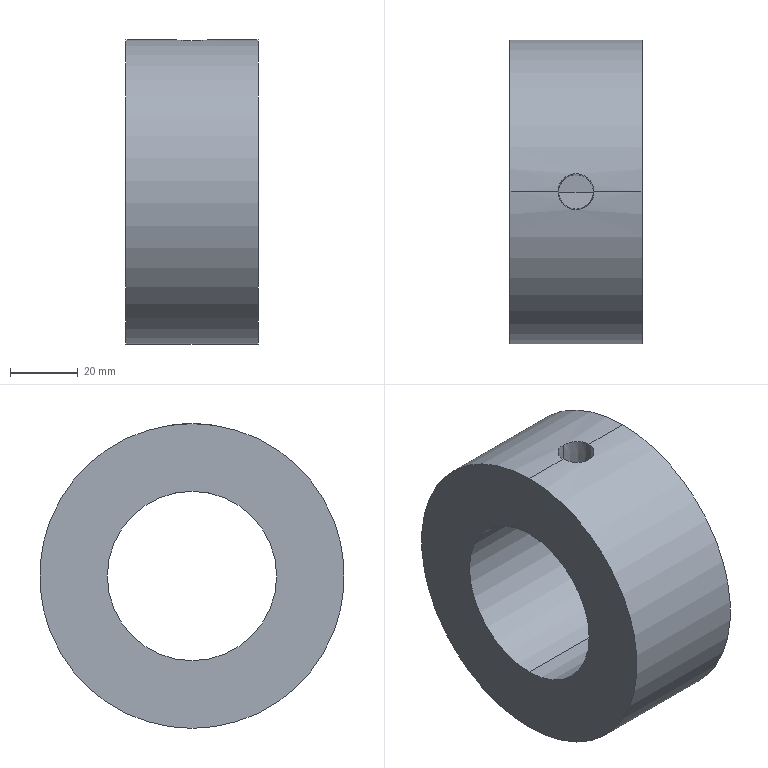Part | SolidWorks | features Extrusion 1, RevCut 1 | 1 solid | 8 faces | box 39 x 90 x 90 mm | volume 169812 mm3 | cylinder 4 | cone 2 | plane 2 | commonest cylinder face diameters 50 x2 90 x2
STEP:
#1=CARTESIAN_POINT('',(147.5,95.12,-78.03));
#2=VERTEX_POINT('',#1);
#3=CARTESIAN_POINT('',(142.375,90.,-77.5));
#4=VERTEX_POINT('',#3);
#5=CARTESIAN_POINT('',(147.5,95.12,-78.03));
#6=CARTESIAN_POINT('',(147.165,95.12,-78.03));
#7=CARTESIAN_POINT('',(146.826,95.086,-78.023));
#8=CARTESIAN_POINT('',(146.167,94.955,-77.996));
#9=CARTESIAN_POINT('',(145.847,94.858,-77.976));
#10=CARTESIAN_POINT('',(145.228,94.601,-77.927));
#11=CARTESIAN_POINT('',(144.928,94.441,-77.897));
#12=CARTESIAN_POINT('',(144.374,94.07,-77.833));
#13=CARTESIAN_POINT('',(144.115,93.859,-77.798));
#14=CARTESIAN_POINT('',(143.638,93.383,-77.729));
#15=CARTESIAN_POINT('',(143.426,93.124,-77.694));
#16=CARTESIAN_POINT('',(143.148,92.709,-77.647));
#17=CARTESIAN_POINT('',(143.062,92.566,-77.632));
#18=CARTESIAN_POINT('',(142.904,92.271,-77.603));
#19=CARTESIAN_POINT('',(142.831,92.117,-77.589));
#20=CARTESIAN_POINT('',(142.637,91.652,-77.553));
#21=CARTESIAN_POINT('',(142.54,91.333,-77.533));
#22=CARTESIAN_POINT('',(142.409,90.676,-77.507));
#23=CARTESIAN_POINT('',(142.375,90.335,-77.5));
#24=CARTESIAN_POINT('',(142.375,90.,-77.5));
#25=B_SPLINE_CURVE_WITH_KNOTS('',3,(#5,#6,#7,#8,#9,#10,#11,#12,#13,#14,#15,#16,#17,#18,#19,#20,#21,#22,#23,#24),.UNSPECIFIED.,.F.,.F.,(4,2,2,2,2,2,2,2,2,4),(0.0199,0.02091,0.02191,0.02292,0.02392,0.02492,0.02542,0.02593,0.02693,0.02793),.UNSPECIFIED.);
#26=EDGE_CURVE('',#2,#4,#25,.T.);
#27=ORIENTED_EDGE('',*,*,#26,.F.);
#28=CARTESIAN_POINT('',(147.5,95.322,-57.816));
#29=VERTEX_POINT('',#28);
#30=CARTESIAN_POINT('',(147.5,95.,-90.));
#31=DIRECTION('',(0.,0.01,1.));
#32=VECTOR('',#31,1000.);
#33=LINE('',#30,#32);
#34=EDGE_CURVE('',#2,#29,#33,.T.);
#35=ORIENTED_EDGE('',*,*,#34,.T.);
#36=CARTESIAN_POINT('',(142.175,90.,-57.5));
#37=VERTEX_POINT('',#36);
#38=CARTESIAN_POINT('',(147.5,95.322,-57.816));
#39=CARTESIAN_POINT('',(147.326,95.322,-57.816));
#40=CARTESIAN_POINT('',(147.153,95.313,-57.815));
#41=CARTESIAN_POINT('',(146.804,95.279,-57.811));
#42=CARTESIAN_POINT('',(146.63,95.253,-57.808));
#43=CARTESIAN_POINT('',(146.116,95.151,-57.796));
#44=CARTESIAN_POINT('',(145.784,95.05,-57.784));
#45=CARTESIAN_POINT('',(145.141,94.784,-57.755));
#46=CARTESIAN_POINT('',(144.829,94.617,-57.737));
#47=CARTESIAN_POINT('',(144.252,94.231,-57.699));
#48=CARTESIAN_POINT('',(143.984,94.012,-57.678));
#49=CARTESIAN_POINT('',(143.488,93.517,-57.637));
#50=CARTESIAN_POINT('',(143.266,93.246,-57.616));
#51=CARTESIAN_POINT('',(142.977,92.814,-57.588));
#52=CARTESIAN_POINT('',(142.888,92.666,-57.579));
#53=CARTESIAN_POINT('',(142.723,92.359,-57.562));
#54=CARTESIAN_POINT('',(142.648,92.2,-57.553));
#55=CARTESIAN_POINT('',(142.447,91.715,-57.532));
#56=CARTESIAN_POINT('',(142.346,91.383,-57.52));
#57=CARTESIAN_POINT('',(142.21,90.701,-57.504));
#58=CARTESIAN_POINT('',(142.175,90.348,-57.5));
#59=CARTESIAN_POINT('',(142.175,90.,-57.5));
#60=B_SPLINE_CURVE_WITH_KNOTS('',3,(#38,#39,#40,#41,#42,#43,#44,#45,#46,#47,#48,#49,#50,#51,#52,#53,#54,#55,#56,#57,#58,#59),.UNSPECIFIED.,.F.,.F.,(4,2,2,2,2,2,2,2,2,2,4),(0.02069,0.02121,0.02173,0.02277,0.02381,0.02485,0.02589,0.02641,0.02694,0.02798,0.02902),.UNSPECIFIED.);
#61=EDGE_CURVE('',#29,#37,#60,.T.);
#62=ORIENTED_EDGE('',*,*,#61,.T.);
#63=CARTESIAN_POINT('',(147.5,84.678,-57.816));
#64=VERTEX_POINT('',#63);
#65=CARTESIAN_POINT('',(142.175,90.,-57.5));
#66=CARTESIAN_POINT('',(142.175,89.652,-57.5));
#67=CARTESIAN_POINT('',(142.209,89.307,-57.504));
#68=CARTESIAN_POINT('',(142.311,88.793,-57.516));
#69=CARTESIAN_POINT('',(142.354,88.622,-57.521));
#70=CARTESIAN_POINT('',(142.455,88.288,-57.532));
#71=CARTESIAN_POINT('',(142.514,88.124,-57.539));
#72=CARTESIAN_POINT('',(142.713,87.644,-57.561));
#73=CARTESIAN_POINT('',(142.876,87.337,-57.578));
#74=CARTESIAN_POINT('',(143.266,86.753,-57.616));
#75=CARTESIAN_POINT('',(143.488,86.483,-57.637));
#76=CARTESIAN_POINT('',(143.983,85.988,-57.678));
#77=CARTESIAN_POINT('',(144.254,85.767,-57.699));
#78=CARTESIAN_POINT('',(144.83,85.382,-57.737));
#79=CARTESIAN_POINT('',(145.14,85.217,-57.755));
#80=CARTESIAN_POINT('',(145.786,84.949,-57.784));
#81=CARTESIAN_POINT('',(146.118,84.849,-57.796));
#82=CARTESIAN_POINT('',(146.799,84.713,-57.812));
#83=CARTESIAN_POINT('',(147.152,84.678,-57.816));
#84=CARTESIAN_POINT('',(147.5,84.678,-57.816));
#85=B_SPLINE_CURVE_WITH_KNOTS('',3,(#65,#66,#67,#68,#69,#70,#71,#72,#73,#74,#75,#76,#77,#78,#79,#80,#81,#82,#83,#84),.UNSPECIFIED.,.F.,.F.,(4,2,2,2,2,2,2,2,2,4),(0.02902,0.03006,0.03058,0.0311,0.03214,0.03318,0.03422,0.03526,0.0363,0.03734),.UNSPECIFIED.);
#86=EDGE_CURVE('',#37,#64,#85,.T.);
#87=ORIENTED_EDGE('',*,*,#86,.T.);
#88=CARTESIAN_POINT('',(147.5,84.88,-78.03));
#89=VERTEX_POINT('',#88);
#90=CARTESIAN_POINT('',(147.5,85.,-90.));
#91=DIRECTION('',(0.,-0.01,1.));
#92=VECTOR('',#91,1000.);
#93=LINE('',#90,#92);
#94=EDGE_CURVE('',#89,#64,#93,.T.);
#95=ORIENTED_EDGE('',*,*,#94,.F.);
#96=CARTESIAN_POINT('',(142.375,90.,-77.5));
#97=CARTESIAN_POINT('',(142.375,89.665,-77.5));
#98=CARTESIAN_POINT('',(142.408,89.332,-77.507));
#99=CARTESIAN_POINT('',(142.506,88.836,-77.527));
#100=CARTESIAN_POINT('',(142.548,88.671,-77.535));
#101=CARTESIAN_POINT('',(142.645,88.35,-77.554));
#102=CARTESIAN_POINT('',(142.702,88.193,-77.565));
#103=CARTESIAN_POINT('',(142.894,87.731,-77.601));
#104=CARTESIAN_POINT('',(143.053,87.434,-77.63));
#105=CARTESIAN_POINT('',(143.427,86.874,-77.695));
#106=CARTESIAN_POINT('',(143.639,86.616,-77.729));
#107=CARTESIAN_POINT('',(144.115,86.141,-77.798));
#108=CARTESIAN_POINT('',(144.376,85.928,-77.833));
#109=CARTESIAN_POINT('',(144.929,85.558,-77.897));
#110=CARTESIAN_POINT('',(145.226,85.399,-77.927));
#111=CARTESIAN_POINT('',(145.849,85.142,-77.976));
#112=CARTESIAN_POINT('',(146.169,85.045,-77.996));
#113=CARTESIAN_POINT('',(146.824,84.914,-78.023));
#114=CARTESIAN_POINT('',(147.164,84.88,-78.03));
#115=CARTESIAN_POINT('',(147.5,84.88,-78.03));
#116=B_SPLINE_CURVE_WITH_KNOTS('',3,(#96,#97,#98,#99,#100,#101,#102,#103,#104,#105,#106,#107,#108,#109,#110,#111,#112,#113,#114,#115),.UNSPECIFIED.,.F.,.F.,(4,2,2,2,2,2,2,2,2,4),(0.02793,0.02894,0.02944,0.02994,0.03094,0.03194,0.03295,0.03395,0.03495,0.03596),.UNSPECIFIED.);
#117=EDGE_CURVE('',#4,#89,#116,.T.);
#118=ORIENTED_EDGE('',*,*,#117,.F.);
#119=EDGE_LOOP('',(#27,#35,#62,#87,#95,#118));
#120=FACE_OUTER_BOUND('',#119,.T.);
#121=CARTESIAN_POINT('',(147.5,90.,-90.));
#122=DIRECTION('',(0.,0.,1.));
#123=DIRECTION('',(0.,-1.,0.));
#124=AXIS2_PLACEMENT_3D('',#121,#122,#123);
#125=CONICAL_SURFACE('',#124,5.,0.01);
#126=ADVANCED_FACE('',(#120),#125,.F.);
#127=CARTESIAN_POINT('',(167.,90.,-127.5));
#128=VERTEX_POINT('',#127);
#129=CARTESIAN_POINT('',(167.,90.,-77.5));
#130=VERTEX_POINT('',#129);
#131=CARTESIAN_POINT('',(167.,90.,-102.5));
#132=DIRECTION('',(-1.,0.,0.));
#133=DIRECTION('',(0.,0.,1.));
#134=AXIS2_PLACEMENT_3D('',#131,#132,#133);
#135=CIRCLE('',#134,25.);
#136=EDGE_CURVE('',#128,#130,#135,.T.);
#137=ORIENTED_EDGE('',*,*,#136,.F.);
#138=CARTESIAN_POINT('',(128.,90.,-127.5));
#139=VERTEX_POINT('',#138);
#140=CARTESIAN_POINT('',(167.,90.,-127.5));
#141=DIRECTION('',(-1.,0.,0.));
#142=VECTOR('',#141,1000.);
#143=LINE('',#140,#142);
#144=EDGE_CURVE('',#128,#139,#143,.T.);
#145=ORIENTED_EDGE('',*,*,#144,.T.);
#146=CARTESIAN_POINT('',(128.,90.,-77.5));
#147=VERTEX_POINT('',#146);
#148=CARTESIAN_POINT('',(128.,90.,-102.5));
#149=DIRECTION('',(-1.,0.,0.));
#150=DIRECTION('',(0.,0.,1.));
#151=AXIS2_PLACEMENT_3D('',#148,#149,#150);
#152=CIRCLE('',#151,25.);
#153=EDGE_CURVE('',#139,#147,#152,.T.);
#154=ORIENTED_EDGE('',*,*,#153,.T.);
#155=CARTESIAN_POINT('',(167.,90.,-77.5));
#156=DIRECTION('',(-1.,0.,0.));
#157=VECTOR('',#156,1000.);
#158=LINE('',#155,#157);
#159=EDGE_CURVE('',#4,#147,#158,.T.);
#160=ORIENTED_EDGE('',*,*,#159,.F.);
#161=ORIENTED_EDGE('',*,*,#117,.T.);
#162=CARTESIAN_POINT('',(152.625,90.,-77.5));
#163=VERTEX_POINT('',#162);
#164=CARTESIAN_POINT('',(147.5,84.88,-78.03));
#165=CARTESIAN_POINT('',(147.836,84.88,-78.03));
#166=CARTESIAN_POINT('',(148.169,84.913,-78.023));
#167=CARTESIAN_POINT('',(148.664,85.011,-78.003));
#168=CARTESIAN_POINT('',(148.829,85.053,-77.994));
#169=CARTESIAN_POINT('',(149.151,85.15,-77.975));
#170=CARTESIAN_POINT('',(149.309,85.207,-77.964));
#171=CARTESIAN_POINT('',(149.772,85.399,-77.927));
#172=CARTESIAN_POINT('',(150.067,85.556,-77.897));
#173=CARTESIAN_POINT('',(150.629,85.931,-77.833));
#174=CARTESIAN_POINT('',(150.887,86.143,-77.798));
#175=CARTESIAN_POINT('',(151.358,86.614,-77.729));
#176=CARTESIAN_POINT('',(151.574,86.876,-77.694));
#177=CARTESIAN_POINT('',(151.947,87.433,-77.631));
#178=CARTESIAN_POINT('',(152.104,87.727,-77.602));
#179=CARTESIAN_POINT('',(152.362,88.345,-77.553));
#180=CARTESIAN_POINT('',(152.461,88.672,-77.533));
#181=CARTESIAN_POINT('',(152.592,89.329,-77.507));
#182=CARTESIAN_POINT('',(152.625,89.662,-77.5));
#183=CARTESIAN_POINT('',(152.625,90.,-77.5));
#184=B_SPLINE_CURVE_WITH_KNOTS('',3,(#164,#165,#166,#167,#168,#169,#170,#171,#172,#173,#174,#175,#176,#177,#178,#179,#180,#181,#182,#183),.UNSPECIFIED.,.F.,.F.,(4,2,2,2,2,2,2,2,2,4),(0.003843,0.004847,0.005349,0.005851,0.006855,0.007859,0.008863,0.009867,0.01087,0.01188),.UNSPECIFIED.);
#185=EDGE_CURVE('',#89,#163,#184,.T.);
#186=ORIENTED_EDGE('',*,*,#185,.T.);
#187=CARTESIAN_POINT('',(167.,90.,-77.5));
#188=DIRECTION('',(-1.,0.,0.));
#189=VECTOR('',#188,1000.);
#190=LINE('',#187,#189);
#191=EDGE_CURVE('',#130,#163,#190,.T.);
#192=ORIENTED_EDGE('',*,*,#191,.F.);
#193=EDGE_LOOP('',(#137,#145,#154,#160,#161,#186,#192));
#194=FACE_OUTER_BOUND('',#193,.T.);
#195=CARTESIAN_POINT('',(167.,90.,-102.5));
#196=DIRECTION('',(-1.,0.,0.));
#197=DIRECTION('',(0.,0.,1.));
#198=AXIS2_PLACEMENT_3D('',#195,#196,#197);
#199=CYLINDRICAL_SURFACE('',#198,25.);
#200=ADVANCED_FACE('',(#194),#199,.F.);
#201=CARTESIAN_POINT('',(167.,90.,-57.5));
#202=VERTEX_POINT('',#201);
#203=CARTESIAN_POINT('',(167.,90.,-147.5));
#204=VERTEX_POINT('',#203);
#205=CARTESIAN_POINT('',(167.,90.,-102.5));
#206=DIRECTION('',(-1.,0.,0.));
#207=DIRECTION('',(0.,0.,1.));
#208=AXIS2_PLACEMENT_3D('',#205,#206,#207);
#209=CIRCLE('',#208,45.);
#210=EDGE_CURVE('',#202,#204,#209,.T.);
#211=ORIENTED_EDGE('',*,*,#210,.T.);
#212=CARTESIAN_POINT('',(128.,90.,-147.5));
#213=VERTEX_POINT('',#212);
#214=CARTESIAN_POINT('',(167.,90.,-147.5));
#215=DIRECTION('',(-1.,0.,0.));
#216=VECTOR('',#215,1000.);
#217=LINE('',#214,#216);
#218=EDGE_CURVE('',#204,#213,#217,.T.);
#219=ORIENTED_EDGE('',*,*,#218,.T.);
#220=CARTESIAN_POINT('',(128.,90.,-57.5));
#221=VERTEX_POINT('',#220);
#222=CARTESIAN_POINT('',(128.,90.,-102.5));
#223=DIRECTION('',(-1.,0.,0.));
#224=DIRECTION('',(0.,0.,1.));
#225=AXIS2_PLACEMENT_3D('',#222,#223,#224);
#226=CIRCLE('',#225,45.);
#227=EDGE_CURVE('',#221,#213,#226,.T.);
#228=ORIENTED_EDGE('',*,*,#227,.F.);
#229=CARTESIAN_POINT('',(167.,90.,-57.5));
#230=DIRECTION('',(-1.,0.,0.));
#231=VECTOR('',#230,1000.);
#232=LINE('',#229,#231);
#233=EDGE_CURVE('',#37,#221,#232,.T.);
#234=ORIENTED_EDGE('',*,*,#233,.F.);
#235=ORIENTED_EDGE('',*,*,#61,.F.);
#236=CARTESIAN_POINT('',(152.825,90.,-57.5));
#237=VERTEX_POINT('',#236);
#238=CARTESIAN_POINT('',(152.825,90.,-57.5));
#239=CARTESIAN_POINT('',(152.825,90.351,-57.5));
#240=CARTESIAN_POINT('',(152.79,90.7,-57.504));
#241=CARTESIAN_POINT('',(152.688,91.21,-57.516));
#242=CARTESIAN_POINT('',(152.646,91.379,-57.521));
#243=CARTESIAN_POINT('',(152.545,91.713,-57.532));
#244=CARTESIAN_POINT('',(152.485,91.879,-57.539));
#245=CARTESIAN_POINT('',(152.284,92.364,-57.561));
#246=CARTESIAN_POINT('',(152.12,92.669,-57.578));
#247=CARTESIAN_POINT('',(151.734,93.246,-57.616));
#248=CARTESIAN_POINT('',(151.509,93.52,-57.637));
#249=CARTESIAN_POINT('',(151.017,94.011,-57.678));
#250=CARTESIAN_POINT('',(150.749,94.231,-57.699));
#251=CARTESIAN_POINT('',(150.314,94.522,-57.728));
#252=CARTESIAN_POINT('',(150.162,94.612,-57.737));
#253=CARTESIAN_POINT('',(149.854,94.777,-57.754));
#254=CARTESIAN_POINT('',(149.697,94.851,-57.762));
#255=CARTESIAN_POINT('',(149.216,95.05,-57.784));
#256=CARTESIAN_POINT('',(148.884,95.151,-57.796));
#257=CARTESIAN_POINT('',(148.193,95.288,-57.812));
#258=CARTESIAN_POINT('',(147.847,95.322,-57.816));
#259=CARTESIAN_POINT('',(147.5,95.322,-57.816));
#260=B_SPLINE_CURVE_WITH_KNOTS('',3,(#238,#239,#240,#241,#242,#243,#244,#245,#246,#247,#248,#249,#250,#251,#252,#253,#254,#255,#256,#257,#258,#259),.UNSPECIFIED.,.F.,.F.,(4,2,2,2,2,2,2,2,2,2,4),(0.01236,0.0134,0.01392,0.01444,0.01548,0.01653,0.01757,0.01809,0.01861,0.01965,0.02069),.UNSPECIFIED.);
#261=EDGE_CURVE('',#237,#29,#260,.T.);
#262=ORIENTED_EDGE('',*,*,#261,.F.);
#263=CARTESIAN_POINT('',(167.,90.,-57.5));
#264=DIRECTION('',(-1.,0.,0.));
#265=VECTOR('',#264,1000.);
#266=LINE('',#263,#265);
#267=EDGE_CURVE('',#202,#237,#266,.T.);
#268=ORIENTED_EDGE('',*,*,#267,.F.);
#269=EDGE_LOOP('',(#211,#219,#228,#234,#235,#262,#268));
#270=FACE_OUTER_BOUND('',#269,.T.);
#271=CARTESIAN_POINT('',(167.,90.,-102.5));
#272=DIRECTION('',(-1.,0.,0.));
#273=DIRECTION('',(0.,0.,1.));
#274=AXIS2_PLACEMENT_3D('',#271,#272,#273);
#275=CYLINDRICAL_SURFACE('',#274,45.);
#276=ADVANCED_FACE('',(#270),#275,.T.);
#277=ORIENTED_EDGE('',*,*,#218,.F.);
#278=CARTESIAN_POINT('',(167.,90.,-102.5));
#279=DIRECTION('',(-1.,0.,0.));
#280=DIRECTION('',(0.,0.,1.));
#281=AXIS2_PLACEMENT_3D('',#278,#279,#280);
#282=CIRCLE('',#281,45.);
#283=EDGE_CURVE('',#204,#202,#282,.T.);
#284=ORIENTED_EDGE('',*,*,#283,.T.);
#285=ORIENTED_EDGE('',*,*,#267,.T.);
#286=CARTESIAN_POINT('',(147.5,84.678,-57.816));
#287=CARTESIAN_POINT('',(147.848,84.678,-57.816));
#288=CARTESIAN_POINT('',(148.194,84.712,-57.812));
#289=CARTESIAN_POINT('',(148.708,84.814,-57.8));
#290=CARTESIAN_POINT('',(148.879,84.857,-57.795));
#291=CARTESIAN_POINT('',(149.214,84.958,-57.783));
#292=CARTESIAN_POINT('',(149.378,85.017,-57.777));
#293=CARTESIAN_POINT('',(149.859,85.216,-57.755));
#294=CARTESIAN_POINT('',(150.166,85.38,-57.737));
#295=CARTESIAN_POINT('',(150.751,85.77,-57.699));
#296=CARTESIAN_POINT('',(151.019,85.991,-57.678));
#297=CARTESIAN_POINT('',(151.387,86.358,-57.647));
#298=CARTESIAN_POINT('',(151.504,86.487,-57.637));
#299=CARTESIAN_POINT('',(151.726,86.757,-57.617));
#300=CARTESIAN_POINT('',(151.831,86.899,-57.607));
#301=CARTESIAN_POINT('',(152.122,87.334,-57.578));
#302=CARTESIAN_POINT('',(152.285,87.639,-57.561));
#303=CARTESIAN_POINT('',(152.552,88.282,-57.532));
#304=CARTESIAN_POINT('',(152.655,88.622,-57.52));
#305=CARTESIAN_POINT('',(152.791,89.304,-57.504));
#306=CARTESIAN_POINT('',(152.825,89.649,-57.5));
#307=CARTESIAN_POINT('',(152.825,90.,-57.5));
#308=B_SPLINE_CURVE_WITH_KNOTS('',3,(#286,#287,#288,#289,#290,#291,#292,#293,#294,#295,#296,#297,#298,#299,#300,#301,#302,#303,#304,#305,#306,#307),.UNSPECIFIED.,.F.,.F.,(4,2,2,2,2,2,2,2,2,2,4),(0.004028,0.005069,0.00559,0.006111,0.007153,0.008194,0.008715,0.009236,0.01028,0.01132,0.01236),.UNSPECIFIED.);
#309=EDGE_CURVE('',#64,#237,#308,.T.);
#310=ORIENTED_EDGE('',*,*,#309,.F.);
#311=ORIENTED_EDGE('',*,*,#86,.F.);
#312=ORIENTED_EDGE('',*,*,#233,.T.);
#313=CARTESIAN_POINT('',(128.,90.,-102.5));
#314=DIRECTION('',(-1.,0.,0.));
#315=DIRECTION('',(0.,0.,1.));
#316=AXIS2_PLACEMENT_3D('',#313,#314,#315);
#317=CIRCLE('',#316,45.);
#318=EDGE_CURVE('',#213,#221,#317,.T.);
#319=ORIENTED_EDGE('',*,*,#318,.F.);
#320=EDGE_LOOP('',(#277,#284,#285,#310,#311,#312,#319));
#321=FACE_OUTER_BOUND('',#320,.T.);
#322=CARTESIAN_POINT('',(167.,90.,-102.5));
#323=DIRECTION('',(-1.,0.,0.));
#324=DIRECTION('',(0.,0.,1.));
#325=AXIS2_PLACEMENT_3D('',#322,#323,#324);
#326=CYLINDRICAL_SURFACE('',#325,45.);
#327=ADVANCED_FACE('',(#321),#326,.T.);
#328=CARTESIAN_POINT('',(167.,90.,-102.5));
#329=DIRECTION('',(-1.,0.,0.));
#330=DIRECTION('',(0.,0.,1.));
#331=AXIS2_PLACEMENT_3D('',#328,#329,#330);
#332=CIRCLE('',#331,25.);
#333=EDGE_CURVE('',#130,#128,#332,.T.);
#334=ORIENTED_EDGE('',*,*,#333,.T.);
#335=ORIENTED_EDGE('',*,*,#136,.T.);
#336=EDGE_LOOP('',(#334,#335));
#337=FACE_BOUND('',#336,.T.);
#338=ORIENTED_EDGE('',*,*,#210,.F.);
#339=ORIENTED_EDGE('',*,*,#283,.F.);
#340=EDGE_LOOP('',(#338,#339));
#341=FACE_OUTER_BOUND('',#340,.T.);
#342=CARTESIAN_POINT('',(167.,90.,-102.5));
#343=DIRECTION('',(-1.,0.,0.));
#344=DIRECTION('',(0.,0.,1.));
#345=AXIS2_PLACEMENT_3D('',#342,#343,#344);
#346=PLANE('',#345);
#347=ADVANCED_FACE('',(#337,#341),#346,.F.);
#348=CARTESIAN_POINT('',(128.,90.,-102.5));
#349=DIRECTION('',(-1.,0.,0.));
#350=DIRECTION('',(0.,0.,1.));
#351=AXIS2_PLACEMENT_3D('',#348,#349,#350);
#352=CIRCLE('',#351,25.);
#353=EDGE_CURVE('',#147,#139,#352,.T.);
#354=ORIENTED_EDGE('',*,*,#353,.F.);
#355=ORIENTED_EDGE('',*,*,#153,.F.);
#356=EDGE_LOOP('',(#354,#355));
#357=FACE_BOUND('',#356,.T.);
#358=ORIENTED_EDGE('',*,*,#227,.T.);
#359=ORIENTED_EDGE('',*,*,#318,.T.);
#360=EDGE_LOOP('',(#358,#359));
#361=FACE_OUTER_BOUND('',#360,.T.);
#362=CARTESIAN_POINT('',(128.,90.,-102.5));
#363=DIRECTION('',(-1.,0.,0.));
#364=DIRECTION('',(0.,0.,1.));
#365=AXIS2_PLACEMENT_3D('',#362,#363,#364);
#366=PLANE('',#365);
#367=ADVANCED_FACE('',(#357,#361),#366,.T.);
#368=ORIENTED_EDGE('',*,*,#144,.F.);
#369=ORIENTED_EDGE('',*,*,#333,.F.);
#370=ORIENTED_EDGE('',*,*,#191,.T.);
#371=CARTESIAN_POINT('',(152.625,90.,-77.5));
#372=CARTESIAN_POINT('',(152.625,90.338,-77.5));
#373=CARTESIAN_POINT('',(152.591,90.675,-77.507));
#374=CARTESIAN_POINT('',(152.493,91.167,-77.527));
#375=CARTESIAN_POINT('',(152.452,91.329,-77.535));
#376=CARTESIAN_POINT('',(152.354,91.65,-77.554));
#377=CARTESIAN_POINT('',(152.297,91.81,-77.565));
#378=CARTESIAN_POINT('',(152.103,92.276,-77.602));
#379=CARTESIAN_POINT('',(151.945,92.57,-77.631));
#380=CARTESIAN_POINT('',(151.573,93.125,-77.695));
#381=CARTESIAN_POINT('',(151.357,93.388,-77.729));
#382=CARTESIAN_POINT('',(150.885,93.859,-77.798));
#383=CARTESIAN_POINT('',(150.627,94.07,-77.833));
#384=CARTESIAN_POINT('',(150.208,94.35,-77.881));
#385=CARTESIAN_POINT('',(150.063,94.437,-77.897));
#386=CARTESIAN_POINT('',(149.767,94.595,-77.926));
#387=CARTESIAN_POINT('',(149.616,94.666,-77.939));
#388=CARTESIAN_POINT('',(149.154,94.857,-77.976));
#389=CARTESIAN_POINT('',(148.832,94.955,-77.996));
#390=CARTESIAN_POINT('',(148.168,95.087,-78.023));
#391=CARTESIAN_POINT('',(147.835,95.12,-78.03));
#392=CARTESIAN_POINT('',(147.5,95.12,-78.03));
#393=B_SPLINE_CURVE_WITH_KNOTS('',3,(#371,#372,#373,#374,#375,#376,#377,#378,#379,#380,#381,#382,#383,#384,#385,#386,#387,#388,#389,#390,#391,#392),.UNSPECIFIED.,.F.,.F.,(4,2,2,2,2,2,2,2,2,2,4),(0.01188,0.01288,0.01338,0.01388,0.01489,0.01589,0.01689,0.0174,0.0179,0.0189,0.0199),.UNSPECIFIED.);
#394=EDGE_CURVE('',#163,#2,#393,.T.);
#395=ORIENTED_EDGE('',*,*,#394,.T.);
#396=ORIENTED_EDGE('',*,*,#26,.T.);
#397=ORIENTED_EDGE('',*,*,#159,.T.);
#398=ORIENTED_EDGE('',*,*,#353,.T.);
#399=EDGE_LOOP('',(#368,#369,#370,#395,#396,#397,#398));
#400=FACE_OUTER_BOUND('',#399,.T.);
#401=CARTESIAN_POINT('',(167.,90.,-102.5));
#402=DIRECTION('',(-1.,0.,0.));
#403=DIRECTION('',(0.,0.,1.));
#404=AXIS2_PLACEMENT_3D('',#401,#402,#403);
#405=CYLINDRICAL_SURFACE('',#404,25.);
#406=ADVANCED_FACE('',(#400),#405,.F.);
#407=ORIENTED_EDGE('',*,*,#34,.F.);
#408=ORIENTED_EDGE('',*,*,#394,.F.);
#409=ORIENTED_EDGE('',*,*,#185,.F.);
#410=ORIENTED_EDGE('',*,*,#94,.T.);
#411=ORIENTED_EDGE('',*,*,#309,.T.);
#412=ORIENTED_EDGE('',*,*,#261,.T.);
#413=EDGE_LOOP('',(#407,#408,#409,#410,#411,#412));
#414=FACE_OUTER_BOUND('',#413,.T.);
#415=CARTESIAN_POINT('',(147.5,90.,-90.));
#416=DIRECTION('',(0.,0.,1.));
#417=DIRECTION('',(0.,-1.,0.));
#418=AXIS2_PLACEMENT_3D('',#415,#416,#417);
#419=CONICAL_SURFACE('',#418,5.,0.01);
#420=ADVANCED_FACE('',(#414),#419,.F.);
#421=CLOSED_SHELL('',(#126,#200,#276,#327,#347,#367,#406,#420));
#422=MANIFOLD_SOLID_BREP('',#421);
#423=CARTESIAN_POINT('',(0.,0.,0.));
#424=DIRECTION('',(0.,0.,1.));
#425=DIRECTION('',(1.,0.,0.));
#426=AXIS2_PLACEMENT_3D('',#423,#424,#425);
#427=(LENGTH_UNIT()NAMED_UNIT(*)SI_UNIT(.MILLI.,.METRE.));
#428=UNCERTAINTY_MEASURE_WITH_UNIT(LENGTH_MEASURE(0.00001),#427,'','');
#429=(NAMED_UNIT(*)PLANE_ANGLE_UNIT()SI_UNIT($,.RADIAN.));
#430=(NAMED_UNIT(*)SI_UNIT($,.STERADIAN.)SOLID_ANGLE_UNIT());
#431=(GEOMETRIC_REPRESENTATION_CONTEXT(3)GLOBAL_UNCERTAINTY_ASSIGNED_CONTEXT((#428))GLOBAL_UNIT_ASSIGNED_CONTEXT((#427,#429,#430))REPRESENTATION_CONTEXT('',''));
#432=ADVANCED_BREP_SHAPE_REPRESENTATION('',(#422,#426),#431);